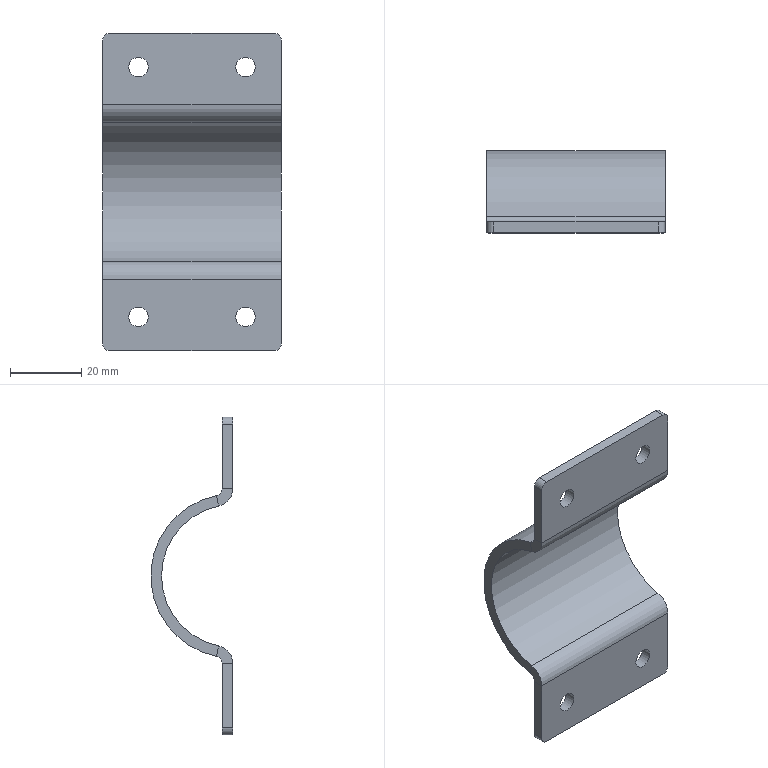Part | NX | 1 solid | 30 faces | box 50 x 23 x 88.99 mm | volume 15975 mm3 | plane 16 | cylinder 14 | commonest cylinder face diameters 4 x6 5.5 x4 10 x2 40 x1 46 x1
STEP:
#1=CARTESIAN_POINT('',(25.,3.,-24.495));
#2=VERTEX_POINT('',#1);
#3=CARTESIAN_POINT('',(25.,0.,-24.495));
#4=VERTEX_POINT('',#3);
#5=CARTESIAN_POINT('',(25.,3.,-24.495));
#6=DIRECTION('',(0.,-1.,0.));
#7=VECTOR('',#6,1000.);
#8=LINE('',#5,#7);
#9=EDGE_CURVE('',#2,#4,#8,.T.);
#10=ORIENTED_EDGE('',*,*,#9,.F.);
#11=CARTESIAN_POINT('',(25.,4.6,-22.535));
#12=VERTEX_POINT('',#11);
#13=CARTESIAN_POINT('',(25.,5.,-24.495));
#14=DIRECTION('',(1.,0.,0.));
#15=DIRECTION('',(0.,0.,-1.));
#16=AXIS2_PLACEMENT_3D('',#13,#14,#15);
#17=CIRCLE('',#16,2.);
#18=EDGE_CURVE('',#2,#12,#17,.F.);
#19=ORIENTED_EDGE('',*,*,#18,.T.);
#20=CARTESIAN_POINT('',(25.,4.,-19.596));
#21=VERTEX_POINT('',#20);
#22=CARTESIAN_POINT('',(25.,4.6,-22.535));
#23=DIRECTION('',(0.,-0.2,0.9798));
#24=VECTOR('',#23,1000.);
#25=LINE('',#22,#24);
#26=EDGE_CURVE('',#12,#21,#25,.T.);
#27=ORIENTED_EDGE('',*,*,#26,.T.);
#28=CARTESIAN_POINT('',(25.,5.,-24.495));
#29=DIRECTION('',(-1.,0.,0.));
#30=DIRECTION('',(0.,0.,1.));
#31=AXIS2_PLACEMENT_3D('',#28,#29,#30);
#32=CIRCLE('',#31,5.);
#33=EDGE_CURVE('',#4,#21,#32,.T.);
#34=ORIENTED_EDGE('',*,*,#33,.F.);
#35=EDGE_LOOP('',(#10,#19,#27,#34));
#36=FACE_BOUND('',#35,.T.);
#37=CARTESIAN_POINT('',(25.,3.,-24.495));
#38=DIRECTION('',(1.,0.,0.));
#39=DIRECTION('',(0.,0.,-1.));
#40=AXIS2_PLACEMENT_3D('',#37,#38,#39);
#41=PLANE('',#40);
#42=ADVANCED_FACE('',(#36),#41,.T.);
#43=CARTESIAN_POINT('',(-25.,0.,-24.495));
#44=VERTEX_POINT('',#43);
#45=CARTESIAN_POINT('',(-25.,3.,-24.495));
#46=VERTEX_POINT('',#45);
#47=CARTESIAN_POINT('',(-25.,0.,-24.495));
#48=DIRECTION('',(0.,1.,0.));
#49=VECTOR('',#48,1000.);
#50=LINE('',#47,#49);
#51=EDGE_CURVE('',#44,#46,#50,.T.);
#52=ORIENTED_EDGE('',*,*,#51,.F.);
#53=CARTESIAN_POINT('',(-25.,4.,-19.596));
#54=VERTEX_POINT('',#53);
#55=CARTESIAN_POINT('',(-25.,5.,-24.495));
#56=DIRECTION('',(-1.,0.,0.));
#57=DIRECTION('',(0.,0.,1.));
#58=AXIS2_PLACEMENT_3D('',#55,#56,#57);
#59=CIRCLE('',#58,5.);
#60=EDGE_CURVE('',#44,#54,#59,.T.);
#61=ORIENTED_EDGE('',*,*,#60,.T.);
#62=CARTESIAN_POINT('',(-25.,4.6,-22.535));
#63=VERTEX_POINT('',#62);
#64=CARTESIAN_POINT('',(-25.,4.,-19.596));
#65=DIRECTION('',(0.,0.2,-0.9798));
#66=VECTOR('',#65,1000.);
#67=LINE('',#64,#66);
#68=EDGE_CURVE('',#54,#63,#67,.T.);
#69=ORIENTED_EDGE('',*,*,#68,.T.);
#70=CARTESIAN_POINT('',(-25.,5.,-24.495));
#71=DIRECTION('',(1.,0.,0.));
#72=DIRECTION('',(0.,0.,-1.));
#73=AXIS2_PLACEMENT_3D('',#70,#71,#72);
#74=CIRCLE('',#73,2.);
#75=EDGE_CURVE('',#46,#63,#74,.F.);
#76=ORIENTED_EDGE('',*,*,#75,.F.);
#77=EDGE_LOOP('',(#52,#61,#69,#76));
#78=FACE_BOUND('',#77,.T.);
#79=CARTESIAN_POINT('',(-25.,0.,-24.495));
#80=DIRECTION('',(-1.,0.,0.));
#81=DIRECTION('',(0.,0.,1.));
#82=AXIS2_PLACEMENT_3D('',#79,#80,#81);
#83=PLANE('',#82);
#84=ADVANCED_FACE('',(#78),#83,.T.);
#85=ORIENTED_EDGE('',*,*,#26,.F.);
#86=CARTESIAN_POINT('',(25.,4.6,22.535));
#87=VERTEX_POINT('',#86);
#88=CARTESIAN_POINT('',(25.,0.,0.));
#89=DIRECTION('',(1.,0.,0.));
#90=DIRECTION('',(0.,0.,-1.));
#91=AXIS2_PLACEMENT_3D('',#88,#89,#90);
#92=CIRCLE('',#91,23.);
#93=EDGE_CURVE('',#12,#87,#92,.T.);
#94=ORIENTED_EDGE('',*,*,#93,.T.);
#95=CARTESIAN_POINT('',(25.,4.,19.596));
#96=VERTEX_POINT('',#95);
#97=CARTESIAN_POINT('',(25.,4.6,22.535));
#98=DIRECTION('',(0.,-0.2,-0.9798));
#99=VECTOR('',#98,1000.);
#100=LINE('',#97,#99);
#101=EDGE_CURVE('',#87,#96,#100,.T.);
#102=ORIENTED_EDGE('',*,*,#101,.T.);
#103=CARTESIAN_POINT('',(25.,0.,0.));
#104=DIRECTION('',(1.,0.,0.));
#105=DIRECTION('',(0.,0.,-1.));
#106=AXIS2_PLACEMENT_3D('',#103,#104,#105);
#107=CIRCLE('',#106,20.);
#108=EDGE_CURVE('',#21,#96,#107,.T.);
#109=ORIENTED_EDGE('',*,*,#108,.F.);
#110=EDGE_LOOP('',(#85,#94,#102,#109));
#111=FACE_BOUND('',#110,.T.);
#112=CARTESIAN_POINT('',(25.,4.6,-22.535));
#113=DIRECTION('',(1.,0.,0.));
#114=DIRECTION('',(0.,0.,-1.));
#115=AXIS2_PLACEMENT_3D('',#112,#113,#114);
#116=PLANE('',#115);
#117=ADVANCED_FACE('',(#111),#116,.T.);
#118=ORIENTED_EDGE('',*,*,#68,.F.);
#119=CARTESIAN_POINT('',(-25.,4.,19.596));
#120=VERTEX_POINT('',#119);
#121=CARTESIAN_POINT('',(-25.,0.,0.));
#122=DIRECTION('',(1.,0.,0.));
#123=DIRECTION('',(0.,0.,-1.));
#124=AXIS2_PLACEMENT_3D('',#121,#122,#123);
#125=CIRCLE('',#124,20.);
#126=EDGE_CURVE('',#54,#120,#125,.T.);
#127=ORIENTED_EDGE('',*,*,#126,.T.);
#128=CARTESIAN_POINT('',(-25.,4.6,22.535));
#129=VERTEX_POINT('',#128);
#130=CARTESIAN_POINT('',(-25.,4.,19.596));
#131=DIRECTION('',(0.,0.2,0.9798));
#132=VECTOR('',#131,1000.);
#133=LINE('',#130,#132);
#134=EDGE_CURVE('',#120,#129,#133,.T.);
#135=ORIENTED_EDGE('',*,*,#134,.T.);
#136=CARTESIAN_POINT('',(-25.,0.,0.));
#137=DIRECTION('',(1.,0.,0.));
#138=DIRECTION('',(0.,0.,-1.));
#139=AXIS2_PLACEMENT_3D('',#136,#137,#138);
#140=CIRCLE('',#139,23.);
#141=EDGE_CURVE('',#63,#129,#140,.T.);
#142=ORIENTED_EDGE('',*,*,#141,.F.);
#143=EDGE_LOOP('',(#118,#127,#135,#142));
#144=FACE_BOUND('',#143,.T.);
#145=CARTESIAN_POINT('',(-25.,4.,-19.596));
#146=DIRECTION('',(-1.,0.,0.));
#147=DIRECTION('',(0.,0.,1.));
#148=AXIS2_PLACEMENT_3D('',#145,#146,#147);
#149=PLANE('',#148);
#150=ADVANCED_FACE('',(#144),#149,.T.);
#151=CARTESIAN_POINT('',(25.,0.,24.495));
#152=VERTEX_POINT('',#151);
#153=CARTESIAN_POINT('',(25.,3.,24.495));
#154=VERTEX_POINT('',#153);
#155=CARTESIAN_POINT('',(25.,0.,24.495));
#156=DIRECTION('',(0.,1.,0.));
#157=VECTOR('',#156,1000.);
#158=LINE('',#155,#157);
#159=EDGE_CURVE('',#152,#154,#158,.T.);
#160=ORIENTED_EDGE('',*,*,#159,.F.);
#161=CARTESIAN_POINT('',(25.,5.,24.495));
#162=DIRECTION('',(-1.,0.,0.));
#163=DIRECTION('',(0.,0.,1.));
#164=AXIS2_PLACEMENT_3D('',#161,#162,#163);
#165=CIRCLE('',#164,5.);
#166=EDGE_CURVE('',#96,#152,#165,.T.);
#167=ORIENTED_EDGE('',*,*,#166,.F.);
#168=ORIENTED_EDGE('',*,*,#101,.F.);
#169=CARTESIAN_POINT('',(25.,5.,24.495));
#170=DIRECTION('',(1.,0.,0.));
#171=DIRECTION('',(0.,0.,-1.));
#172=AXIS2_PLACEMENT_3D('',#169,#170,#171);
#173=CIRCLE('',#172,2.);
#174=EDGE_CURVE('',#87,#154,#173,.F.);
#175=ORIENTED_EDGE('',*,*,#174,.T.);
#176=EDGE_LOOP('',(#160,#167,#168,#175));
#177=FACE_BOUND('',#176,.T.);
#178=CARTESIAN_POINT('',(25.,0.,24.495));
#179=DIRECTION('',(1.,0.,0.));
#180=DIRECTION('',(0.,0.,-1.));
#181=AXIS2_PLACEMENT_3D('',#178,#179,#180);
#182=PLANE('',#181);
#183=ADVANCED_FACE('',(#177),#182,.T.);
#184=CARTESIAN_POINT('',(25.,3.,42.495));
#185=VERTEX_POINT('',#184);
#186=CARTESIAN_POINT('',(25.,3.,24.495));
#187=DIRECTION('',(0.,0.,1.));
#188=VECTOR('',#187,1000.);
#189=LINE('',#186,#188);
#190=EDGE_CURVE('',#154,#185,#189,.T.);
#191=ORIENTED_EDGE('',*,*,#190,.T.);
#192=CARTESIAN_POINT('',(25.,0.,42.495));
#193=VERTEX_POINT('',#192);
#194=CARTESIAN_POINT('',(25.,4.6,42.495));
#195=DIRECTION('',(0.,1.,0.));
#196=VECTOR('',#195,1000.);
#197=LINE('',#194,#196);
#198=EDGE_CURVE('',#185,#193,#197,.F.);
#199=ORIENTED_EDGE('',*,*,#198,.T.);
#200=CARTESIAN_POINT('',(25.,0.,24.495));
#201=DIRECTION('',(0.,0.,1.));
#202=VECTOR('',#201,1000.);
#203=LINE('',#200,#202);
#204=EDGE_CURVE('',#152,#193,#203,.T.);
#205=ORIENTED_EDGE('',*,*,#204,.F.);
#206=ORIENTED_EDGE('',*,*,#159,.T.);
#207=EDGE_LOOP('',(#191,#199,#205,#206));
#208=FACE_BOUND('',#207,.T.);
#209=CARTESIAN_POINT('',(25.,4.6,22.535));
#210=DIRECTION('',(1.,0.,0.));
#211=DIRECTION('',(0.,0.,-1.));
#212=AXIS2_PLACEMENT_3D('',#209,#210,#211);
#213=PLANE('',#212);
#214=ADVANCED_FACE('',(#208),#213,.T.);
#215=ORIENTED_EDGE('',*,*,#134,.F.);
#216=CARTESIAN_POINT('',(-25.,0.,24.495));
#217=VERTEX_POINT('',#216);
#218=CARTESIAN_POINT('',(-25.,5.,24.495));
#219=DIRECTION('',(-1.,0.,0.));
#220=DIRECTION('',(0.,0.,1.));
#221=AXIS2_PLACEMENT_3D('',#218,#219,#220);
#222=CIRCLE('',#221,5.);
#223=EDGE_CURVE('',#120,#217,#222,.T.);
#224=ORIENTED_EDGE('',*,*,#223,.T.);
#225=CARTESIAN_POINT('',(-25.,3.,24.495));
#226=VERTEX_POINT('',#225);
#227=CARTESIAN_POINT('',(-25.,3.,24.495));
#228=DIRECTION('',(0.,-1.,0.));
#229=VECTOR('',#228,1000.);
#230=LINE('',#227,#229);
#231=EDGE_CURVE('',#226,#217,#230,.T.);
#232=ORIENTED_EDGE('',*,*,#231,.F.);
#233=CARTESIAN_POINT('',(-25.,5.,24.495));
#234=DIRECTION('',(1.,0.,0.));
#235=DIRECTION('',(0.,0.,-1.));
#236=AXIS2_PLACEMENT_3D('',#233,#234,#235);
#237=CIRCLE('',#236,2.);
#238=EDGE_CURVE('',#129,#226,#237,.F.);
#239=ORIENTED_EDGE('',*,*,#238,.F.);
#240=EDGE_LOOP('',(#215,#224,#232,#239));
#241=FACE_BOUND('',#240,.T.);
#242=CARTESIAN_POINT('',(-25.,4.,19.596));
#243=DIRECTION('',(-1.,0.,0.));
#244=DIRECTION('',(0.,0.,1.));
#245=AXIS2_PLACEMENT_3D('',#242,#243,#244);
#246=PLANE('',#245);
#247=ADVANCED_FACE('',(#241),#246,.T.);
#248=CARTESIAN_POINT('',(-25.,3.,-42.495));
#249=VERTEX_POINT('',#248);
#250=CARTESIAN_POINT('',(-25.,3.,-24.495));
#251=DIRECTION('',(0.,0.,1.));
#252=VECTOR('',#251,1000.);
#253=LINE('',#250,#252);
#254=EDGE_CURVE('',#249,#46,#253,.T.);
#255=ORIENTED_EDGE('',*,*,#254,.F.);
#256=CARTESIAN_POINT('',(-25.,0.,-42.495));
#257=VERTEX_POINT('',#256);
#258=CARTESIAN_POINT('',(-25.,3.,-42.495));
#259=DIRECTION('',(0.,-1.,0.));
#260=VECTOR('',#259,1000.);
#261=LINE('',#258,#260);
#262=EDGE_CURVE('',#249,#257,#261,.T.);
#263=ORIENTED_EDGE('',*,*,#262,.T.);
#264=CARTESIAN_POINT('',(-25.,0.,-24.495));
#265=DIRECTION('',(0.,0.,1.));
#266=VECTOR('',#265,1000.);
#267=LINE('',#264,#266);
#268=EDGE_CURVE('',#257,#44,#267,.T.);
#269=ORIENTED_EDGE('',*,*,#268,.T.);
#270=ORIENTED_EDGE('',*,*,#51,.T.);
#271=EDGE_LOOP('',(#255,#263,#269,#270));
#272=FACE_BOUND('',#271,.T.);
#273=CARTESIAN_POINT('',(-25.,3.,24.495));
#274=DIRECTION('',(-1.,0.,0.));
#275=DIRECTION('',(0.,0.,1.));
#276=AXIS2_PLACEMENT_3D('',#273,#274,#275);
#277=PLANE('',#276);
#278=ADVANCED_FACE('',(#272),#277,.T.);
#279=CARTESIAN_POINT('',(15.,3.,37.75));
#280=VERTEX_POINT('',#279);
#281=CARTESIAN_POINT('',(15.,3.,35.));
#282=DIRECTION('',(0.,1.,0.));
#283=DIRECTION('',(0.,0.,1.));
#284=AXIS2_PLACEMENT_3D('',#281,#282,#283);
#285=CIRCLE('',#284,2.75);
#286=EDGE_CURVE('',#280,#280,#285,.T.);
#287=ORIENTED_EDGE('',*,*,#286,.F.);
#288=EDGE_LOOP('',(#287));
#289=FACE_BOUND('',#288,.T.);
#290=CARTESIAN_POINT('',(-15.,3.,37.75));
#291=VERTEX_POINT('',#290);
#292=CARTESIAN_POINT('',(-15.,3.,35.));
#293=DIRECTION('',(0.,1.,0.));
#294=DIRECTION('',(0.,0.,1.));
#295=AXIS2_PLACEMENT_3D('',#292,#293,#294);
#296=CIRCLE('',#295,2.75);
#297=EDGE_CURVE('',#291,#291,#296,.T.);
#298=ORIENTED_EDGE('',*,*,#297,.F.);
#299=EDGE_LOOP('',(#298));
#300=FACE_BOUND('',#299,.T.);
#301=CARTESIAN_POINT('',(-25.,3.,42.495));
#302=VERTEX_POINT('',#301);
#303=CARTESIAN_POINT('',(-25.,3.,24.495));
#304=DIRECTION('',(0.,0.,1.));
#305=VECTOR('',#304,1000.);
#306=LINE('',#303,#305);
#307=EDGE_CURVE('',#226,#302,#306,.T.);
#308=ORIENTED_EDGE('',*,*,#307,.T.);
#309=CARTESIAN_POINT('',(-23.,3.,44.495));
#310=VERTEX_POINT('',#309);
#311=CARTESIAN_POINT('',(-23.,3.,42.495));
#312=DIRECTION('',(0.,-1.,0.));
#313=DIRECTION('',(0.,0.,-1.));
#314=AXIS2_PLACEMENT_3D('',#311,#312,#313);
#315=CIRCLE('',#314,2.);
#316=EDGE_CURVE('',#302,#310,#315,.F.);
#317=ORIENTED_EDGE('',*,*,#316,.T.);
#318=CARTESIAN_POINT('',(23.,3.,44.495));
#319=VERTEX_POINT('',#318);
#320=CARTESIAN_POINT('',(25.,3.,44.495));
#321=DIRECTION('',(-1.,0.,0.));
#322=VECTOR('',#321,1000.);
#323=LINE('',#320,#322);
#324=EDGE_CURVE('',#319,#310,#323,.T.);
#325=ORIENTED_EDGE('',*,*,#324,.F.);
#326=CARTESIAN_POINT('',(23.,3.,42.495));
#327=DIRECTION('',(0.,-1.,0.));
#328=DIRECTION('',(0.,0.,-1.));
#329=AXIS2_PLACEMENT_3D('',#326,#327,#328);
#330=CIRCLE('',#329,2.);
#331=EDGE_CURVE('',#319,#185,#330,.F.);
#332=ORIENTED_EDGE('',*,*,#331,.T.);
#333=ORIENTED_EDGE('',*,*,#190,.F.);
#334=CARTESIAN_POINT('',(25.,3.,24.495));
#335=DIRECTION('',(-1.,0.,0.));
#336=VECTOR('',#335,1000.);
#337=LINE('',#334,#336);
#338=EDGE_CURVE('',#154,#226,#337,.T.);
#339=ORIENTED_EDGE('',*,*,#338,.T.);
#340=EDGE_LOOP('',(#308,#317,#325,#332,#333,#339));
#341=FACE_BOUND('',#340,.T.);
#342=CARTESIAN_POINT('',(25.,3.,24.495));
#343=DIRECTION('',(0.,-1.,0.));
#344=DIRECTION('',(0.,0.,-1.));
#345=AXIS2_PLACEMENT_3D('',#342,#343,#344);
#346=PLANE('',#345);
#347=ADVANCED_FACE('',(#289,#300,#341),#346,.F.);
#348=ORIENTED_EDGE('',*,*,#324,.T.);
#349=CARTESIAN_POINT('',(-23.,0.,44.495));
#350=VERTEX_POINT('',#349);
#351=CARTESIAN_POINT('',(-23.,0.,44.495));
#352=DIRECTION('',(0.,1.,0.));
#353=VECTOR('',#352,1000.);
#354=LINE('',#351,#353);
#355=EDGE_CURVE('',#310,#350,#354,.F.);
#356=ORIENTED_EDGE('',*,*,#355,.T.);
#357=CARTESIAN_POINT('',(23.,0.,44.495));
#358=VERTEX_POINT('',#357);
#359=CARTESIAN_POINT('',(25.,0.,44.495));
#360=DIRECTION('',(-1.,0.,0.));
#361=VECTOR('',#360,1000.);
#362=LINE('',#359,#361);
#363=EDGE_CURVE('',#358,#350,#362,.T.);
#364=ORIENTED_EDGE('',*,*,#363,.F.);
#365=CARTESIAN_POINT('',(23.,0.,44.495));
#366=DIRECTION('',(0.,1.,0.));
#367=VECTOR('',#366,1000.);
#368=LINE('',#365,#367);
#369=EDGE_CURVE('',#358,#319,#368,.T.);
#370=ORIENTED_EDGE('',*,*,#369,.T.);
#371=EDGE_LOOP('',(#348,#356,#364,#370));
#372=FACE_BOUND('',#371,.T.);
#373=CARTESIAN_POINT('',(25.,0.,44.495));
#374=DIRECTION('',(0.,0.,1.));
#375=DIRECTION('',(1.,0.,0.));
#376=AXIS2_PLACEMENT_3D('',#373,#374,#375);
#377=PLANE('',#376);
#378=ADVANCED_FACE('',(#372),#377,.T.);
#379=CARTESIAN_POINT('',(15.,0.,37.75));
#380=VERTEX_POINT('',#379);
#381=CARTESIAN_POINT('',(15.,0.,35.));
#382=DIRECTION('',(0.,1.,0.));
#383=DIRECTION('',(0.,0.,1.));
#384=AXIS2_PLACEMENT_3D('',#381,#382,#383);
#385=CIRCLE('',#384,2.75);
#386=EDGE_CURVE('',#380,#380,#385,.T.);
#387=ORIENTED_EDGE('',*,*,#386,.T.);
#388=EDGE_LOOP('',(#387));
#389=FACE_BOUND('',#388,.T.);
#390=CARTESIAN_POINT('',(-15.,0.,37.75));
#391=VERTEX_POINT('',#390);
#392=CARTESIAN_POINT('',(-15.,0.,35.));
#393=DIRECTION('',(0.,1.,0.));
#394=DIRECTION('',(0.,0.,1.));
#395=AXIS2_PLACEMENT_3D('',#392,#393,#394);
#396=CIRCLE('',#395,2.75);
#397=EDGE_CURVE('',#391,#391,#396,.T.);
#398=ORIENTED_EDGE('',*,*,#397,.T.);
#399=EDGE_LOOP('',(#398));
#400=FACE_BOUND('',#399,.T.);
#401=ORIENTED_EDGE('',*,*,#363,.T.);
#402=CARTESIAN_POINT('',(-25.,0.,42.495));
#403=VERTEX_POINT('',#402);
#404=CARTESIAN_POINT('',(-23.,0.,42.495));
#405=DIRECTION('',(0.,-1.,0.));
#406=DIRECTION('',(0.,0.,-1.));
#407=AXIS2_PLACEMENT_3D('',#404,#405,#406);
#408=CIRCLE('',#407,2.);
#409=EDGE_CURVE('',#350,#403,#408,.T.);
#410=ORIENTED_EDGE('',*,*,#409,.T.);
#411=CARTESIAN_POINT('',(-25.,0.,24.495));
#412=DIRECTION('',(0.,0.,1.));
#413=VECTOR('',#412,1000.);
#414=LINE('',#411,#413);
#415=EDGE_CURVE('',#217,#403,#414,.T.);
#416=ORIENTED_EDGE('',*,*,#415,.F.);
#417=CARTESIAN_POINT('',(25.,0.,24.495));
#418=DIRECTION('',(-1.,0.,0.));
#419=VECTOR('',#418,1000.);
#420=LINE('',#417,#419);
#421=EDGE_CURVE('',#152,#217,#420,.T.);
#422=ORIENTED_EDGE('',*,*,#421,.F.);
#423=ORIENTED_EDGE('',*,*,#204,.T.);
#424=CARTESIAN_POINT('',(23.,0.,42.495));
#425=DIRECTION('',(0.,-1.,0.));
#426=DIRECTION('',(0.,0.,-1.));
#427=AXIS2_PLACEMENT_3D('',#424,#425,#426);
#428=CIRCLE('',#427,2.);
#429=EDGE_CURVE('',#193,#358,#428,.T.);
#430=ORIENTED_EDGE('',*,*,#429,.T.);
#431=EDGE_LOOP('',(#401,#410,#416,#422,#423,#430));
#432=FACE_BOUND('',#431,.T.);
#433=CARTESIAN_POINT('',(25.,0.,24.495));
#434=DIRECTION('',(0.,-1.,0.));
#435=DIRECTION('',(0.,0.,-1.));
#436=AXIS2_PLACEMENT_3D('',#433,#434,#435);
#437=PLANE('',#436);
#438=ADVANCED_FACE('',(#389,#400,#432),#437,.T.);
#439=ORIENTED_EDGE('',*,*,#223,.F.);
#440=CARTESIAN_POINT('',(25.,4.,19.596));
#441=DIRECTION('',(-1.,0.,0.));
#442=VECTOR('',#441,1000.);
#443=LINE('',#440,#442);
#444=EDGE_CURVE('',#96,#120,#443,.T.);
#445=ORIENTED_EDGE('',*,*,#444,.F.);
#446=ORIENTED_EDGE('',*,*,#166,.T.);
#447=ORIENTED_EDGE('',*,*,#421,.T.);
#448=EDGE_LOOP('',(#439,#445,#446,#447));
#449=FACE_BOUND('',#448,.T.);
#450=CARTESIAN_POINT('',(25.,5.,24.495));
#451=DIRECTION('',(-1.,0.,0.));
#452=DIRECTION('',(0.,0.,1.));
#453=AXIS2_PLACEMENT_3D('',#450,#451,#452);
#454=CYLINDRICAL_SURFACE('',#453,5.);
#455=ADVANCED_FACE('',(#449),#454,.T.);
#456=ORIENTED_EDGE('',*,*,#126,.F.);
#457=CARTESIAN_POINT('',(25.,4.,-19.596));
#458=DIRECTION('',(-1.,0.,0.));
#459=VECTOR('',#458,1000.);
#460=LINE('',#457,#459);
#461=EDGE_CURVE('',#21,#54,#460,.T.);
#462=ORIENTED_EDGE('',*,*,#461,.F.);
#463=ORIENTED_EDGE('',*,*,#108,.T.);
#464=ORIENTED_EDGE('',*,*,#444,.T.);
#465=EDGE_LOOP('',(#456,#462,#463,#464));
#466=FACE_BOUND('',#465,.T.);
#467=CARTESIAN_POINT('',(25.,0.,0.));
#468=DIRECTION('',(-1.,0.,0.));
#469=DIRECTION('',(0.,0.,1.));
#470=AXIS2_PLACEMENT_3D('',#467,#468,#469);
#471=CYLINDRICAL_SURFACE('',#470,20.);
#472=ADVANCED_FACE('',(#466),#471,.F.);
#473=ORIENTED_EDGE('',*,*,#60,.F.);
#474=CARTESIAN_POINT('',(25.,0.,-24.495));
#475=DIRECTION('',(-1.,0.,0.));
#476=VECTOR('',#475,1000.);
#477=LINE('',#474,#476);
#478=EDGE_CURVE('',#4,#44,#477,.T.);
#479=ORIENTED_EDGE('',*,*,#478,.F.);
#480=ORIENTED_EDGE('',*,*,#33,.T.);
#481=ORIENTED_EDGE('',*,*,#461,.T.);
#482=EDGE_LOOP('',(#473,#479,#480,#481));
#483=FACE_BOUND('',#482,.T.);
#484=CARTESIAN_POINT('',(25.,5.,-24.495));
#485=DIRECTION('',(-1.,0.,0.));
#486=DIRECTION('',(0.,0.,1.));
#487=AXIS2_PLACEMENT_3D('',#484,#485,#486);
#488=CYLINDRICAL_SURFACE('',#487,5.);
#489=ADVANCED_FACE('',(#483),#488,.T.);
#490=CARTESIAN_POINT('',(15.,0.,-32.25));
#491=VERTEX_POINT('',#490);
#492=CARTESIAN_POINT('',(15.,0.,-35.));
#493=DIRECTION('',(0.,1.,0.));
#494=DIRECTION('',(0.,0.,1.));
#495=AXIS2_PLACEMENT_3D('',#492,#493,#494);
#496=CIRCLE('',#495,2.75);
#497=EDGE_CURVE('',#491,#491,#496,.T.);
#498=ORIENTED_EDGE('',*,*,#497,.T.);
#499=EDGE_LOOP('',(#498));
#500=FACE_BOUND('',#499,.T.);
#501=CARTESIAN_POINT('',(-15.,0.,-32.25));
#502=VERTEX_POINT('',#501);
#503=CARTESIAN_POINT('',(-15.,0.,-35.));
#504=DIRECTION('',(0.,1.,0.));
#505=DIRECTION('',(0.,0.,1.));
#506=AXIS2_PLACEMENT_3D('',#503,#504,#505);
#507=CIRCLE('',#506,2.75);
#508=EDGE_CURVE('',#502,#502,#507,.T.);
#509=ORIENTED_EDGE('',*,*,#508,.T.);
#510=EDGE_LOOP('',(#509));
#511=FACE_BOUND('',#510,.T.);
#512=CARTESIAN_POINT('',(23.,0.,-44.495));
#513=VERTEX_POINT('',#512);
#514=CARTESIAN_POINT('',(-23.,0.,-44.495));
#515=VERTEX_POINT('',#514);
#516=CARTESIAN_POINT('',(25.,0.,-44.495));
#517=DIRECTION('',(-1.,0.,0.));
#518=VECTOR('',#517,1000.);
#519=LINE('',#516,#518);
#520=EDGE_CURVE('',#513,#515,#519,.T.);
#521=ORIENTED_EDGE('',*,*,#520,.F.);
#522=CARTESIAN_POINT('',(25.,0.,-42.495));
#523=VERTEX_POINT('',#522);
#524=CARTESIAN_POINT('',(23.,0.,-42.495));
#525=DIRECTION('',(0.,-1.,0.));
#526=DIRECTION('',(0.,0.,-1.));
#527=AXIS2_PLACEMENT_3D('',#524,#525,#526);
#528=CIRCLE('',#527,2.);
#529=EDGE_CURVE('',#513,#523,#528,.T.);
#530=ORIENTED_EDGE('',*,*,#529,.T.);
#531=CARTESIAN_POINT('',(25.,0.,-24.495));
#532=DIRECTION('',(0.,0.,1.));
#533=VECTOR('',#532,1000.);
#534=LINE('',#531,#533);
#535=EDGE_CURVE('',#523,#4,#534,.T.);
#536=ORIENTED_EDGE('',*,*,#535,.T.);
#537=ORIENTED_EDGE('',*,*,#478,.T.);
#538=ORIENTED_EDGE('',*,*,#268,.F.);
#539=CARTESIAN_POINT('',(-23.,0.,-42.495));
#540=DIRECTION('',(0.,-1.,0.));
#541=DIRECTION('',(0.,0.,-1.));
#542=AXIS2_PLACEMENT_3D('',#539,#540,#541);
#543=CIRCLE('',#542,2.);
#544=EDGE_CURVE('',#257,#515,#543,.T.);
#545=ORIENTED_EDGE('',*,*,#544,.T.);
#546=EDGE_LOOP('',(#521,#530,#536,#537,#538,#545));
#547=FACE_BOUND('',#546,.T.);
#548=CARTESIAN_POINT('',(25.,0.,-24.495));
#549=DIRECTION('',(0.,-1.,0.));
#550=DIRECTION('',(0.,0.,-1.));
#551=AXIS2_PLACEMENT_3D('',#548,#549,#550);
#552=PLANE('',#551);
#553=ADVANCED_FACE('',(#500,#511,#547),#552,.T.);
#554=CARTESIAN_POINT('',(23.,3.,-44.495));
#555=VERTEX_POINT('',#554);
#556=CARTESIAN_POINT('',(-23.,3.,-44.495));
#557=VERTEX_POINT('',#556);
#558=CARTESIAN_POINT('',(25.,3.,-44.495));
#559=DIRECTION('',(-1.,0.,0.));
#560=VECTOR('',#559,1000.);
#561=LINE('',#558,#560);
#562=EDGE_CURVE('',#555,#557,#561,.T.);
#563=ORIENTED_EDGE('',*,*,#562,.F.);
#564=CARTESIAN_POINT('',(23.,0.,-44.495));
#565=DIRECTION('',(0.,-1.,0.));
#566=VECTOR('',#565,1000.);
#567=LINE('',#564,#566);
#568=EDGE_CURVE('',#555,#513,#567,.T.);
#569=ORIENTED_EDGE('',*,*,#568,.T.);
#570=ORIENTED_EDGE('',*,*,#520,.T.);
#571=CARTESIAN_POINT('',(-23.,3.,-44.495));
#572=DIRECTION('',(0.,-1.,0.));
#573=VECTOR('',#572,1000.);
#574=LINE('',#571,#573);
#575=EDGE_CURVE('',#515,#557,#574,.F.);
#576=ORIENTED_EDGE('',*,*,#575,.T.);
#577=EDGE_LOOP('',(#563,#569,#570,#576));
#578=FACE_BOUND('',#577,.T.);
#579=CARTESIAN_POINT('',(25.,3.,-44.495));
#580=DIRECTION('',(0.,0.,-1.));
#581=DIRECTION('',(-1.,0.,0.));
#582=AXIS2_PLACEMENT_3D('',#579,#580,#581);
#583=PLANE('',#582);
#584=ADVANCED_FACE('',(#578),#583,.T.);
#585=CARTESIAN_POINT('',(15.,3.,-32.25));
#586=VERTEX_POINT('',#585);
#587=CARTESIAN_POINT('',(15.,3.,-35.));
#588=DIRECTION('',(0.,1.,0.));
#589=DIRECTION('',(0.,0.,1.));
#590=AXIS2_PLACEMENT_3D('',#587,#588,#589);
#591=CIRCLE('',#590,2.75);
#592=EDGE_CURVE('',#586,#586,#591,.T.);
#593=ORIENTED_EDGE('',*,*,#592,.F.);
#594=EDGE_LOOP('',(#593));
#595=FACE_BOUND('',#594,.T.);
#596=CARTESIAN_POINT('',(-15.,3.,-32.25));
#597=VERTEX_POINT('',#596);
#598=CARTESIAN_POINT('',(-15.,3.,-35.));
#599=DIRECTION('',(0.,1.,0.));
#600=DIRECTION('',(0.,0.,1.));
#601=AXIS2_PLACEMENT_3D('',#598,#599,#600);
#602=CIRCLE('',#601,2.75);
#603=EDGE_CURVE('',#597,#597,#602,.T.);
#604=ORIENTED_EDGE('',*,*,#603,.F.);
#605=EDGE_LOOP('',(#604));
#606=FACE_BOUND('',#605,.T.);
#607=CARTESIAN_POINT('',(25.,3.,-42.495));
#608=VERTEX_POINT('',#607);
#609=CARTESIAN_POINT('',(25.,3.,-24.495));
#610=DIRECTION('',(0.,0.,1.));
#611=VECTOR('',#610,1000.);
#612=LINE('',#609,#611);
#613=EDGE_CURVE('',#608,#2,#612,.T.);
#614=ORIENTED_EDGE('',*,*,#613,.F.);
#615=CARTESIAN_POINT('',(23.,3.,-42.495));
#616=DIRECTION('',(0.,-1.,0.));
#617=DIRECTION('',(0.,0.,-1.));
#618=AXIS2_PLACEMENT_3D('',#615,#616,#617);
#619=CIRCLE('',#618,2.);
#620=EDGE_CURVE('',#608,#555,#619,.F.);
#621=ORIENTED_EDGE('',*,*,#620,.T.);
#622=ORIENTED_EDGE('',*,*,#562,.T.);
#623=CARTESIAN_POINT('',(-23.,3.,-42.495));
#624=DIRECTION('',(0.,-1.,0.));
#625=DIRECTION('',(0.,0.,-1.));
#626=AXIS2_PLACEMENT_3D('',#623,#624,#625);
#627=CIRCLE('',#626,2.);
#628=EDGE_CURVE('',#557,#249,#627,.F.);
#629=ORIENTED_EDGE('',*,*,#628,.T.);
#630=ORIENTED_EDGE('',*,*,#254,.T.);
#631=CARTESIAN_POINT('',(25.,3.,-24.495));
#632=DIRECTION('',(-1.,0.,0.));
#633=VECTOR('',#632,1000.);
#634=LINE('',#631,#633);
#635=EDGE_CURVE('',#2,#46,#634,.T.);
#636=ORIENTED_EDGE('',*,*,#635,.F.);
#637=EDGE_LOOP('',(#614,#621,#622,#629,#630,#636));
#638=FACE_BOUND('',#637,.T.);
#639=CARTESIAN_POINT('',(25.,3.,-24.495));
#640=DIRECTION('',(0.,-1.,0.));
#641=DIRECTION('',(0.,0.,-1.));
#642=AXIS2_PLACEMENT_3D('',#639,#640,#641);
#643=PLANE('',#642);
#644=ADVANCED_FACE('',(#595,#606,#638),#643,.F.);
#645=ORIENTED_EDGE('',*,*,#75,.T.);
#646=CARTESIAN_POINT('',(25.,4.6,-22.535));
#647=DIRECTION('',(-1.,0.,0.));
#648=VECTOR('',#647,1000.);
#649=LINE('',#646,#648);
#650=EDGE_CURVE('',#12,#63,#649,.T.);
#651=ORIENTED_EDGE('',*,*,#650,.F.);
#652=ORIENTED_EDGE('',*,*,#18,.F.);
#653=ORIENTED_EDGE('',*,*,#635,.T.);
#654=EDGE_LOOP('',(#645,#651,#652,#653));
#655=FACE_BOUND('',#654,.T.);
#656=CARTESIAN_POINT('',(25.,5.,-24.495));
#657=DIRECTION('',(-1.,0.,0.));
#658=DIRECTION('',(0.,0.,1.));
#659=AXIS2_PLACEMENT_3D('',#656,#657,#658);
#660=CYLINDRICAL_SURFACE('',#659,2.);
#661=ADVANCED_FACE('',(#655),#660,.F.);
#662=ORIENTED_EDGE('',*,*,#141,.T.);
#663=CARTESIAN_POINT('',(25.,4.6,22.535));
#664=DIRECTION('',(-1.,0.,0.));
#665=VECTOR('',#664,1000.);
#666=LINE('',#663,#665);
#667=EDGE_CURVE('',#87,#129,#666,.T.);
#668=ORIENTED_EDGE('',*,*,#667,.F.);
#669=ORIENTED_EDGE('',*,*,#93,.F.);
#670=ORIENTED_EDGE('',*,*,#650,.T.);
#671=EDGE_LOOP('',(#662,#668,#669,#670));
#672=FACE_BOUND('',#671,.T.);
#673=CARTESIAN_POINT('',(25.,0.,0.));
#674=DIRECTION('',(-1.,0.,0.));
#675=DIRECTION('',(0.,0.,1.));
#676=AXIS2_PLACEMENT_3D('',#673,#674,#675);
#677=CYLINDRICAL_SURFACE('',#676,23.);
#678=ADVANCED_FACE('',(#672),#677,.T.);
#679=ORIENTED_EDGE('',*,*,#238,.T.);
#680=ORIENTED_EDGE('',*,*,#338,.F.);
#681=ORIENTED_EDGE('',*,*,#174,.F.);
#682=ORIENTED_EDGE('',*,*,#667,.T.);
#683=EDGE_LOOP('',(#679,#680,#681,#682));
#684=FACE_BOUND('',#683,.T.);
#685=CARTESIAN_POINT('',(25.,5.,24.495));
#686=DIRECTION('',(-1.,0.,0.));
#687=DIRECTION('',(0.,0.,1.));
#688=AXIS2_PLACEMENT_3D('',#685,#686,#687);
#689=CYLINDRICAL_SURFACE('',#688,2.);
#690=ADVANCED_FACE('',(#684),#689,.F.);
#691=ORIENTED_EDGE('',*,*,#535,.F.);
#692=CARTESIAN_POINT('',(25.,3.,-42.495));
#693=DIRECTION('',(0.,-1.,0.));
#694=VECTOR('',#693,1000.);
#695=LINE('',#692,#694);
#696=EDGE_CURVE('',#523,#608,#695,.F.);
#697=ORIENTED_EDGE('',*,*,#696,.T.);
#698=ORIENTED_EDGE('',*,*,#613,.T.);
#699=ORIENTED_EDGE('',*,*,#9,.T.);
#700=EDGE_LOOP('',(#691,#697,#698,#699));
#701=FACE_BOUND('',#700,.T.);
#702=CARTESIAN_POINT('',(25.,5.,24.495));
#703=DIRECTION('',(-1.,0.,0.));
#704=DIRECTION('',(0.,0.,1.));
#705=AXIS2_PLACEMENT_3D('',#702,#703,#704);
#706=PLANE('',#705);
#707=ADVANCED_FACE('',(#701),#706,.F.);
#708=ORIENTED_EDGE('',*,*,#415,.T.);
#709=CARTESIAN_POINT('',(-25.,5.,42.495));
#710=DIRECTION('',(0.,1.,0.));
#711=VECTOR('',#710,1000.);
#712=LINE('',#709,#711);
#713=EDGE_CURVE('',#403,#302,#712,.T.);
#714=ORIENTED_EDGE('',*,*,#713,.T.);
#715=ORIENTED_EDGE('',*,*,#307,.F.);
#716=ORIENTED_EDGE('',*,*,#231,.T.);
#717=EDGE_LOOP('',(#708,#714,#715,#716));
#718=FACE_BOUND('',#717,.T.);
#719=CARTESIAN_POINT('',(-25.,5.,24.495));
#720=DIRECTION('',(-1.,0.,0.));
#721=DIRECTION('',(0.,0.,1.));
#722=AXIS2_PLACEMENT_3D('',#719,#720,#721);
#723=PLANE('',#722);
#724=ADVANCED_FACE('',(#718),#723,.T.);
#725=ORIENTED_EDGE('',*,*,#508,.F.);
#726=EDGE_LOOP('',(#725));
#727=FACE_BOUND('',#726,.T.);
#728=ORIENTED_EDGE('',*,*,#603,.T.);
#729=EDGE_LOOP('',(#728));
#730=FACE_BOUND('',#729,.T.);
#731=CARTESIAN_POINT('',(-15.,3.,-35.));
#732=DIRECTION('',(0.,1.,0.));
#733=DIRECTION('',(0.,0.,1.));
#734=AXIS2_PLACEMENT_3D('',#731,#732,#733);
#735=CYLINDRICAL_SURFACE('',#734,2.75);
#736=ADVANCED_FACE('',(#727,#730),#735,.F.);
#737=ORIENTED_EDGE('',*,*,#397,.F.);
#738=EDGE_LOOP('',(#737));
#739=FACE_BOUND('',#738,.T.);
#740=ORIENTED_EDGE('',*,*,#297,.T.);
#741=EDGE_LOOP('',(#740));
#742=FACE_BOUND('',#741,.T.);
#743=CARTESIAN_POINT('',(-15.,3.,35.));
#744=DIRECTION('',(0.,1.,0.));
#745=DIRECTION('',(0.,0.,1.));
#746=AXIS2_PLACEMENT_3D('',#743,#744,#745);
#747=CYLINDRICAL_SURFACE('',#746,2.75);
#748=ADVANCED_FACE('',(#739,#742),#747,.F.);
#749=ORIENTED_EDGE('',*,*,#386,.F.);
#750=EDGE_LOOP('',(#749));
#751=FACE_BOUND('',#750,.T.);
#752=ORIENTED_EDGE('',*,*,#286,.T.);
#753=EDGE_LOOP('',(#752));
#754=FACE_BOUND('',#753,.T.);
#755=CARTESIAN_POINT('',(15.,3.,35.));
#756=DIRECTION('',(0.,1.,0.));
#757=DIRECTION('',(0.,0.,1.));
#758=AXIS2_PLACEMENT_3D('',#755,#756,#757);
#759=CYLINDRICAL_SURFACE('',#758,2.75);
#760=ADVANCED_FACE('',(#751,#754),#759,.F.);
#761=ORIENTED_EDGE('',*,*,#497,.F.);
#762=EDGE_LOOP('',(#761));
#763=FACE_BOUND('',#762,.T.);
#764=ORIENTED_EDGE('',*,*,#592,.T.);
#765=EDGE_LOOP('',(#764));
#766=FACE_BOUND('',#765,.T.);
#767=CARTESIAN_POINT('',(15.,3.,-35.));
#768=DIRECTION('',(0.,1.,0.));
#769=DIRECTION('',(0.,0.,1.));
#770=AXIS2_PLACEMENT_3D('',#767,#768,#769);
#771=CYLINDRICAL_SURFACE('',#770,2.75);
#772=ADVANCED_FACE('',(#763,#766),#771,.F.);
#773=ORIENTED_EDGE('',*,*,#620,.F.);
#774=ORIENTED_EDGE('',*,*,#696,.F.);
#775=ORIENTED_EDGE('',*,*,#529,.F.);
#776=ORIENTED_EDGE('',*,*,#568,.F.);
#777=EDGE_LOOP('',(#773,#774,#775,#776));
#778=FACE_BOUND('',#777,.T.);
#779=CARTESIAN_POINT('',(23.,3.,-42.495));
#780=DIRECTION('',(0.,1.,0.));
#781=DIRECTION('',(0.,0.,1.));
#782=AXIS2_PLACEMENT_3D('',#779,#780,#781);
#783=CYLINDRICAL_SURFACE('',#782,2.);
#784=ADVANCED_FACE('',(#778),#783,.T.);
#785=ORIENTED_EDGE('',*,*,#628,.F.);
#786=ORIENTED_EDGE('',*,*,#575,.F.);
#787=ORIENTED_EDGE('',*,*,#544,.F.);
#788=ORIENTED_EDGE('',*,*,#262,.F.);
#789=EDGE_LOOP('',(#785,#786,#787,#788));
#790=FACE_BOUND('',#789,.T.);
#791=CARTESIAN_POINT('',(-23.,3.,-42.495));
#792=DIRECTION('',(0.,-1.,0.));
#793=DIRECTION('',(0.,0.,-1.));
#794=AXIS2_PLACEMENT_3D('',#791,#792,#793);
#795=CYLINDRICAL_SURFACE('',#794,2.);
#796=ADVANCED_FACE('',(#790),#795,.T.);
#797=ORIENTED_EDGE('',*,*,#409,.F.);
#798=ORIENTED_EDGE('',*,*,#355,.F.);
#799=ORIENTED_EDGE('',*,*,#316,.F.);
#800=ORIENTED_EDGE('',*,*,#713,.F.);
#801=EDGE_LOOP('',(#797,#798,#799,#800));
#802=FACE_BOUND('',#801,.T.);
#803=CARTESIAN_POINT('',(-23.,5.,42.495));
#804=DIRECTION('',(0.,1.,0.));
#805=DIRECTION('',(0.,0.,1.));
#806=AXIS2_PLACEMENT_3D('',#803,#804,#805);
#807=CYLINDRICAL_SURFACE('',#806,2.);
#808=ADVANCED_FACE('',(#802),#807,.T.);
#809=ORIENTED_EDGE('',*,*,#429,.F.);
#810=ORIENTED_EDGE('',*,*,#198,.F.);
#811=ORIENTED_EDGE('',*,*,#331,.F.);
#812=ORIENTED_EDGE('',*,*,#369,.F.);
#813=EDGE_LOOP('',(#809,#810,#811,#812));
#814=FACE_BOUND('',#813,.T.);
#815=CARTESIAN_POINT('',(23.,0.,42.495));
#816=DIRECTION('',(0.,1.,0.));
#817=DIRECTION('',(0.,0.,1.));
#818=AXIS2_PLACEMENT_3D('',#815,#816,#817);
#819=CYLINDRICAL_SURFACE('',#818,2.);
#820=ADVANCED_FACE('',(#814),#819,.T.);
#821=CLOSED_SHELL('',(#42,#84,#117,#150,#183,#214,#247,#278,#347,#378,#438,#455,#472,#489,#553,#584,#644,#661,#678,#690,#707,#724,#736,#748,#760,#772,#784,#796,#808,#820));
#822=MANIFOLD_SOLID_BREP('',#821);
#823=(LENGTH_UNIT()NAMED_UNIT(*)SI_UNIT(.MILLI.,.METRE.));
#824=UNCERTAINTY_MEASURE_WITH_UNIT(LENGTH_MEASURE(0.00001),#823,'','');
#825=(NAMED_UNIT(*)PLANE_ANGLE_UNIT()SI_UNIT($,.RADIAN.));
#826=(NAMED_UNIT(*)SI_UNIT($,.STERADIAN.)SOLID_ANGLE_UNIT());
#827=(GEOMETRIC_REPRESENTATION_CONTEXT(3)GLOBAL_UNCERTAINTY_ASSIGNED_CONTEXT((#824))GLOBAL_UNIT_ASSIGNED_CONTEXT((#823,#825,#826))REPRESENTATION_CONTEXT('',''));
#828=ADVANCED_BREP_SHAPE_REPRESENTATION('',(#822),#827);